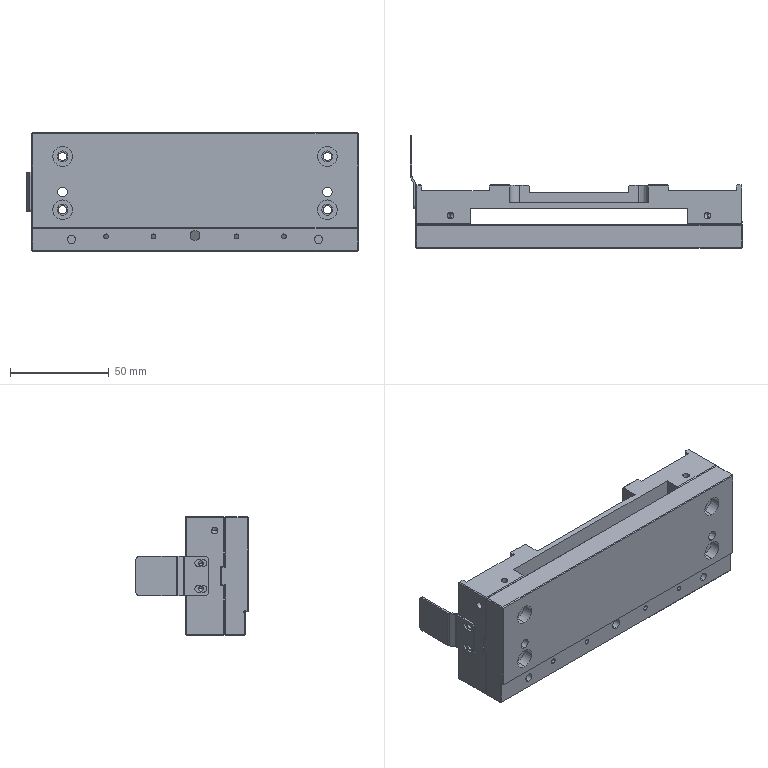Part | SolidWorks | 3 solids | 320 faces | box 168.001 x 57 x 60 mm | volume 203187 mm3 | plane 173 | cylinder 128 | cone 19 | commonest cylinder face diameters 4.5 x24 8 x24 2.5 x16 4.2 x12 5 x12 10 x10